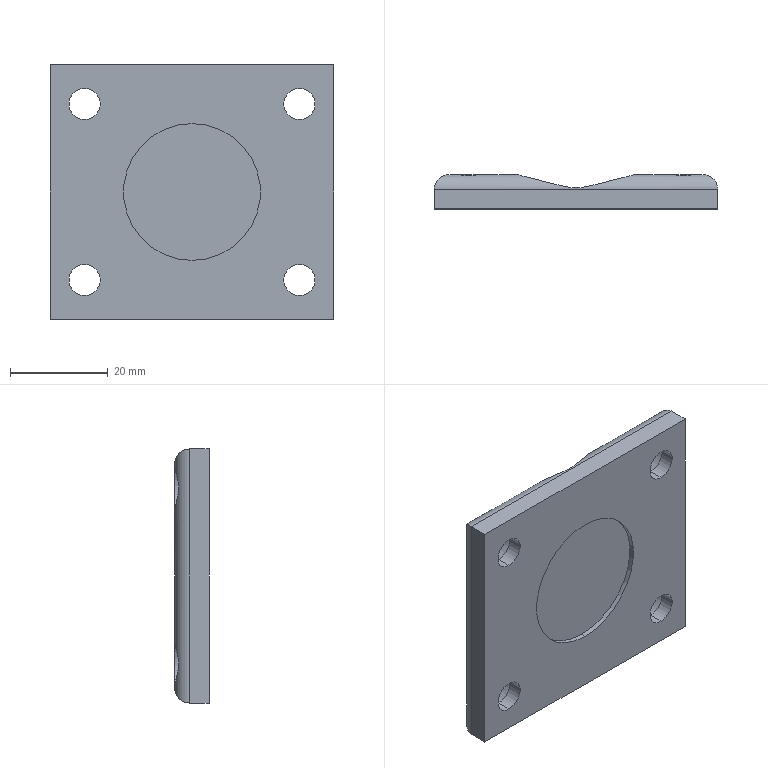Part | NX | features BREP 1 | 1 solid | 41 faces | box 58 x 7 x 52 mm | volume 16120 mm3 | cylinder 23 | plane 18 | commonest cylinder face diameters 6.4 x8 12 x8 6 x4 28 x2 20 x1
STEP:
#1=CARTESIAN_POINT('',(0.,204.,14.));
#2=VERTEX_POINT('',#1);
#3=CARTESIAN_POINT('',(0.,204.,-14.));
#4=VERTEX_POINT('',#3);
#5=CARTESIAN_POINT('',(0.,204.,0.));
#6=DIRECTION('',(0.,-1.,0.));
#7=DIRECTION('',(0.,0.,-1.));
#8=AXIS2_PLACEMENT_3D('',#5,#6,#7);
#9=CIRCLE('',#8,14.);
#10=EDGE_CURVE('',#2,#4,#9,.T.);
#11=ORIENTED_EDGE('',*,*,#10,.F.);
#12=CARTESIAN_POINT('',(0.,203.,14.));
#13=VERTEX_POINT('',#12);
#14=CARTESIAN_POINT('',(0.,204.,14.));
#15=DIRECTION('',(0.,-1.,0.));
#16=VECTOR('',#15,1000.);
#17=LINE('',#14,#16);
#18=EDGE_CURVE('',#2,#13,#17,.T.);
#19=ORIENTED_EDGE('',*,*,#18,.T.);
#20=CARTESIAN_POINT('',(0.,203.,-14.));
#21=VERTEX_POINT('',#20);
#22=CARTESIAN_POINT('',(0.,203.,0.));
#23=DIRECTION('',(0.,-1.,0.));
#24=DIRECTION('',(0.,0.,-1.));
#25=AXIS2_PLACEMENT_3D('',#22,#23,#24);
#26=CIRCLE('',#25,14.);
#27=EDGE_CURVE('',#13,#21,#26,.T.);
#28=ORIENTED_EDGE('',*,*,#27,.T.);
#29=CARTESIAN_POINT('',(0.,204.,-14.));
#30=DIRECTION('',(0.,1.,0.));
#31=VECTOR('',#30,1000.);
#32=LINE('',#29,#31);
#33=EDGE_CURVE('',#21,#4,#32,.T.);
#34=ORIENTED_EDGE('',*,*,#33,.T.);
#35=EDGE_LOOP('',(#11,#19,#28,#34));
#36=FACE_BOUND('',#35,.T.);
#37=CARTESIAN_POINT('',(0.,204.,0.));
#38=DIRECTION('',(0.,-1.,0.));
#39=DIRECTION('',(0.,0.,1.));
#40=AXIS2_PLACEMENT_3D('',#37,#38,#39);
#41=CYLINDRICAL_SURFACE('',#40,14.);
#42=ADVANCED_FACE('',(#36),#41,.F.);
#43=CARTESIAN_POINT('',(-22.,206.,-24.));
#44=VERTEX_POINT('',#43);
#45=CARTESIAN_POINT('',(-22.,206.,-12.));
#46=VERTEX_POINT('',#45);
#47=CARTESIAN_POINT('',(-22.,206.,-18.));
#48=DIRECTION('',(0.,1.,0.));
#49=DIRECTION('',(0.,0.,1.));
#50=AXIS2_PLACEMENT_3D('',#47,#48,#49);
#51=CIRCLE('',#50,6.);
#52=EDGE_CURVE('',#44,#46,#51,.T.);
#53=ORIENTED_EDGE('',*,*,#52,.F.);
#54=CARTESIAN_POINT('',(-22.,209.828,-24.));
#55=VERTEX_POINT('',#54);
#56=CARTESIAN_POINT('',(-22.,206.,-24.));
#57=DIRECTION('',(0.,1.,0.));
#58=VECTOR('',#57,1000.);
#59=LINE('',#56,#58);
#60=EDGE_CURVE('',#44,#55,#59,.T.);
#61=ORIENTED_EDGE('',*,*,#60,.T.);
#62=CARTESIAN_POINT('',(-25.317,210.,-23.));
#63=VERTEX_POINT('',#62);
#64=CARTESIAN_POINT('',(-22.,209.828,-24.));
#65=CARTESIAN_POINT('',(-23.183,209.828,-24.));
#66=CARTESIAN_POINT('',(-24.331,210.,-23.654));
#67=CARTESIAN_POINT('',(-25.317,210.,-23.));
#68=B_SPLINE_CURVE_WITH_KNOTS('',3,(#64,#65,#66,#67),.UNSPECIFIED.,.F.,.F.,(4,4),(0.,0.003498),.UNSPECIFIED.);
#69=EDGE_CURVE('',#55,#63,#68,.T.);
#70=ORIENTED_EDGE('',*,*,#69,.T.);
#71=CARTESIAN_POINT('',(-26.,210.,-22.472));
#72=VERTEX_POINT('',#71);
#73=CARTESIAN_POINT('',(-22.,210.,-18.));
#74=DIRECTION('',(0.,1.,0.));
#75=DIRECTION('',(0.,0.,1.));
#76=AXIS2_PLACEMENT_3D('',#73,#74,#75);
#77=CIRCLE('',#76,6.);
#78=EDGE_CURVE('',#63,#72,#77,.T.);
#79=ORIENTED_EDGE('',*,*,#78,.T.);
#80=CARTESIAN_POINT('',(-26.,210.,-13.528));
#81=VERTEX_POINT('',#80);
#82=CARTESIAN_POINT('',(-26.,210.,-22.472));
#83=CARTESIAN_POINT('',(-26.643,210.,-21.897));
#84=CARTESIAN_POINT('',(-27.633,209.605,-20.529));
#85=CARTESIAN_POINT('',(-28.183,209.052,-18.004));
#86=CARTESIAN_POINT('',(-27.634,209.604,-15.471));
#87=CARTESIAN_POINT('',(-26.642,210.,-14.102));
#88=CARTESIAN_POINT('',(-26.,210.,-13.528));
#89=B_SPLINE_CURVE_WITH_KNOTS('',3,(#82,#83,#84,#85,#86,#87,#88),.UNSPECIFIED.,.F.,.F.,(4,1,1,1,4),(0.,0.00255,0.0051,0.00765,0.0102),.UNSPECIFIED.);
#90=EDGE_CURVE('',#72,#81,#89,.T.);
#91=ORIENTED_EDGE('',*,*,#90,.T.);
#92=CARTESIAN_POINT('',(-22.,210.,-12.));
#93=VERTEX_POINT('',#92);
#94=CARTESIAN_POINT('',(-22.,210.,-18.));
#95=DIRECTION('',(0.,1.,0.));
#96=DIRECTION('',(0.,0.,1.));
#97=AXIS2_PLACEMENT_3D('',#94,#95,#96);
#98=CIRCLE('',#97,6.);
#99=EDGE_CURVE('',#81,#93,#98,.T.);
#100=ORIENTED_EDGE('',*,*,#99,.T.);
#101=CARTESIAN_POINT('',(-22.,206.,-12.));
#102=DIRECTION('',(0.,-1.,0.));
#103=VECTOR('',#102,1000.);
#104=LINE('',#101,#103);
#105=EDGE_CURVE('',#93,#46,#104,.T.);
#106=ORIENTED_EDGE('',*,*,#105,.T.);
#107=EDGE_LOOP('',(#53,#61,#70,#79,#91,#100,#106));
#108=FACE_BOUND('',#107,.T.);
#109=CARTESIAN_POINT('',(-22.,206.,-18.));
#110=DIRECTION('',(0.,1.,0.));
#111=DIRECTION('',(0.,0.,-1.));
#112=AXIS2_PLACEMENT_3D('',#109,#110,#111);
#113=CYLINDRICAL_SURFACE('',#112,6.);
#114=ADVANCED_FACE('',(#108),#113,.F.);
#115=CARTESIAN_POINT('',(22.,206.,-24.));
#116=VERTEX_POINT('',#115);
#117=CARTESIAN_POINT('',(22.,206.,-12.));
#118=VERTEX_POINT('',#117);
#119=CARTESIAN_POINT('',(22.,206.,-18.));
#120=DIRECTION('',(0.,1.,0.));
#121=DIRECTION('',(0.,0.,1.));
#122=AXIS2_PLACEMENT_3D('',#119,#120,#121);
#123=CIRCLE('',#122,6.);
#124=EDGE_CURVE('',#116,#118,#123,.T.);
#125=ORIENTED_EDGE('',*,*,#124,.F.);
#126=CARTESIAN_POINT('',(22.,209.828,-24.));
#127=VERTEX_POINT('',#126);
#128=CARTESIAN_POINT('',(22.,206.,-24.));
#129=DIRECTION('',(0.,-1.,0.));
#130=VECTOR('',#129,1000.);
#131=LINE('',#128,#130);
#132=EDGE_CURVE('',#127,#116,#131,.T.);
#133=ORIENTED_EDGE('',*,*,#132,.F.);
#134=CARTESIAN_POINT('',(18.683,210.,-23.));
#135=VERTEX_POINT('',#134);
#136=CARTESIAN_POINT('',(22.,209.828,-24.));
#137=CARTESIAN_POINT('',(20.817,209.828,-24.));
#138=CARTESIAN_POINT('',(19.669,210.,-23.654));
#139=CARTESIAN_POINT('',(18.683,210.,-23.));
#140=B_SPLINE_CURVE_WITH_KNOTS('',3,(#136,#137,#138,#139),.UNSPECIFIED.,.F.,.F.,(4,4),(0.,0.003498),.UNSPECIFIED.);
#141=EDGE_CURVE('',#127,#135,#140,.T.);
#142=ORIENTED_EDGE('',*,*,#141,.T.);
#143=CARTESIAN_POINT('',(22.,210.,-12.));
#144=VERTEX_POINT('',#143);
#145=CARTESIAN_POINT('',(22.,210.,-18.));
#146=DIRECTION('',(0.,1.,0.));
#147=DIRECTION('',(0.,0.,1.));
#148=AXIS2_PLACEMENT_3D('',#145,#146,#147);
#149=CIRCLE('',#148,6.);
#150=EDGE_CURVE('',#135,#144,#149,.T.);
#151=ORIENTED_EDGE('',*,*,#150,.T.);
#152=CARTESIAN_POINT('',(22.,206.,-12.));
#153=DIRECTION('',(0.,1.,0.));
#154=VECTOR('',#153,1000.);
#155=LINE('',#152,#154);
#156=EDGE_CURVE('',#118,#144,#155,.T.);
#157=ORIENTED_EDGE('',*,*,#156,.F.);
#158=EDGE_LOOP('',(#125,#133,#142,#151,#157));
#159=FACE_BOUND('',#158,.T.);
#160=CARTESIAN_POINT('',(22.,206.,-18.));
#161=DIRECTION('',(0.,1.,0.));
#162=DIRECTION('',(0.,0.,-1.));
#163=AXIS2_PLACEMENT_3D('',#160,#161,#162);
#164=CYLINDRICAL_SURFACE('',#163,6.);
#165=ADVANCED_FACE('',(#159),#164,.F.);
#166=CARTESIAN_POINT('',(22.,206.,12.));
#167=VERTEX_POINT('',#166);
#168=CARTESIAN_POINT('',(22.,206.,24.));
#169=VERTEX_POINT('',#168);
#170=CARTESIAN_POINT('',(22.,206.,18.));
#171=DIRECTION('',(0.,1.,0.));
#172=DIRECTION('',(0.,0.,1.));
#173=AXIS2_PLACEMENT_3D('',#170,#171,#172);
#174=CIRCLE('',#173,6.);
#175=EDGE_CURVE('',#167,#169,#174,.T.);
#176=ORIENTED_EDGE('',*,*,#175,.F.);
#177=CARTESIAN_POINT('',(22.,210.,12.));
#178=VERTEX_POINT('',#177);
#179=CARTESIAN_POINT('',(22.,206.,12.));
#180=DIRECTION('',(0.,1.,0.));
#181=VECTOR('',#180,1000.);
#182=LINE('',#179,#181);
#183=EDGE_CURVE('',#167,#178,#182,.T.);
#184=ORIENTED_EDGE('',*,*,#183,.T.);
#185=CARTESIAN_POINT('',(18.683,210.,23.));
#186=VERTEX_POINT('',#185);
#187=CARTESIAN_POINT('',(22.,210.,18.));
#188=DIRECTION('',(0.,1.,0.));
#189=DIRECTION('',(0.,0.,1.));
#190=AXIS2_PLACEMENT_3D('',#187,#188,#189);
#191=CIRCLE('',#190,6.);
#192=EDGE_CURVE('',#178,#186,#191,.T.);
#193=ORIENTED_EDGE('',*,*,#192,.T.);
#194=CARTESIAN_POINT('',(22.,209.828,24.));
#195=VERTEX_POINT('',#194);
#196=CARTESIAN_POINT('',(18.683,210.,23.));
#197=CARTESIAN_POINT('',(19.67,210.,23.654));
#198=CARTESIAN_POINT('',(20.818,209.828,24.));
#199=CARTESIAN_POINT('',(22.,209.828,24.));
#200=B_SPLINE_CURVE_WITH_KNOTS('',3,(#196,#197,#198,#199),.UNSPECIFIED.,.F.,.F.,(4,4),(0.,0.003499),.UNSPECIFIED.);
#201=EDGE_CURVE('',#186,#195,#200,.T.);
#202=ORIENTED_EDGE('',*,*,#201,.T.);
#203=CARTESIAN_POINT('',(22.,206.,24.));
#204=DIRECTION('',(0.,-1.,0.));
#205=VECTOR('',#204,1000.);
#206=LINE('',#203,#205);
#207=EDGE_CURVE('',#195,#169,#206,.T.);
#208=ORIENTED_EDGE('',*,*,#207,.T.);
#209=EDGE_LOOP('',(#176,#184,#193,#202,#208));
#210=FACE_BOUND('',#209,.T.);
#211=CARTESIAN_POINT('',(22.,206.,18.));
#212=DIRECTION('',(0.,1.,0.));
#213=DIRECTION('',(0.,0.,-1.));
#214=AXIS2_PLACEMENT_3D('',#211,#212,#213);
#215=CYLINDRICAL_SURFACE('',#214,6.);
#216=ADVANCED_FACE('',(#210),#215,.F.);
#217=CARTESIAN_POINT('',(-22.,206.,12.));
#218=VERTEX_POINT('',#217);
#219=CARTESIAN_POINT('',(-22.,206.,24.));
#220=VERTEX_POINT('',#219);
#221=CARTESIAN_POINT('',(-22.,206.,18.));
#222=DIRECTION('',(0.,1.,0.));
#223=DIRECTION('',(0.,0.,1.));
#224=AXIS2_PLACEMENT_3D('',#221,#222,#223);
#225=CIRCLE('',#224,6.);
#226=EDGE_CURVE('',#218,#220,#225,.T.);
#227=ORIENTED_EDGE('',*,*,#226,.F.);
#228=CARTESIAN_POINT('',(-22.,210.,12.));
#229=VERTEX_POINT('',#228);
#230=CARTESIAN_POINT('',(-22.,206.,12.));
#231=DIRECTION('',(0.,1.,0.));
#232=VECTOR('',#231,1000.);
#233=LINE('',#230,#232);
#234=EDGE_CURVE('',#218,#229,#233,.T.);
#235=ORIENTED_EDGE('',*,*,#234,.T.);
#236=CARTESIAN_POINT('',(-26.,210.,13.528));
#237=VERTEX_POINT('',#236);
#238=CARTESIAN_POINT('',(-22.,210.,18.));
#239=DIRECTION('',(0.,1.,0.));
#240=DIRECTION('',(0.,0.,1.));
#241=AXIS2_PLACEMENT_3D('',#238,#239,#240);
#242=CIRCLE('',#241,6.);
#243=EDGE_CURVE('',#229,#237,#242,.T.);
#244=ORIENTED_EDGE('',*,*,#243,.T.);
#245=CARTESIAN_POINT('',(-26.,210.,22.472));
#246=VERTEX_POINT('',#245);
#247=CARTESIAN_POINT('',(-26.,210.,13.528));
#248=CARTESIAN_POINT('',(-26.643,210.,14.103));
#249=CARTESIAN_POINT('',(-27.633,209.605,15.471));
#250=CARTESIAN_POINT('',(-28.183,209.052,17.996));
#251=CARTESIAN_POINT('',(-27.634,209.604,20.529));
#252=CARTESIAN_POINT('',(-26.642,210.,21.898));
#253=CARTESIAN_POINT('',(-26.,210.,22.472));
#254=B_SPLINE_CURVE_WITH_KNOTS('',3,(#247,#248,#249,#250,#251,#252,#253),.UNSPECIFIED.,.F.,.F.,(4,1,1,1,4),(0.,0.00255,0.0051,0.00765,0.0102),.UNSPECIFIED.);
#255=EDGE_CURVE('',#237,#246,#254,.T.);
#256=ORIENTED_EDGE('',*,*,#255,.T.);
#257=CARTESIAN_POINT('',(-25.317,210.,23.));
#258=VERTEX_POINT('',#257);
#259=CARTESIAN_POINT('',(-22.,210.,18.));
#260=DIRECTION('',(0.,1.,0.));
#261=DIRECTION('',(0.,0.,1.));
#262=AXIS2_PLACEMENT_3D('',#259,#260,#261);
#263=CIRCLE('',#262,6.);
#264=EDGE_CURVE('',#246,#258,#263,.T.);
#265=ORIENTED_EDGE('',*,*,#264,.T.);
#266=CARTESIAN_POINT('',(-22.,209.828,24.));
#267=VERTEX_POINT('',#266);
#268=CARTESIAN_POINT('',(-25.317,210.,23.));
#269=CARTESIAN_POINT('',(-24.33,210.,23.654));
#270=CARTESIAN_POINT('',(-23.182,209.828,24.));
#271=CARTESIAN_POINT('',(-22.,209.828,24.));
#272=B_SPLINE_CURVE_WITH_KNOTS('',3,(#268,#269,#270,#271),.UNSPECIFIED.,.F.,.F.,(4,4),(0.,0.003499),.UNSPECIFIED.);
#273=EDGE_CURVE('',#258,#267,#272,.T.);
#274=ORIENTED_EDGE('',*,*,#273,.T.);
#275=CARTESIAN_POINT('',(-22.,206.,24.));
#276=DIRECTION('',(0.,-1.,0.));
#277=VECTOR('',#276,1000.);
#278=LINE('',#275,#277);
#279=EDGE_CURVE('',#267,#220,#278,.T.);
#280=ORIENTED_EDGE('',*,*,#279,.T.);
#281=EDGE_LOOP('',(#227,#235,#244,#256,#265,#274,#280));
#282=FACE_BOUND('',#281,.T.);
#283=CARTESIAN_POINT('',(-22.,206.,18.));
#284=DIRECTION('',(0.,1.,0.));
#285=DIRECTION('',(0.,0.,-1.));
#286=AXIS2_PLACEMENT_3D('',#283,#284,#285);
#287=CYLINDRICAL_SURFACE('',#286,6.);
#288=ADVANCED_FACE('',(#282),#287,.F.);
#289=CARTESIAN_POINT('',(-22.,206.,14.8));
#290=VERTEX_POINT('',#289);
#291=CARTESIAN_POINT('',(-22.,206.,21.2));
#292=VERTEX_POINT('',#291);
#293=CARTESIAN_POINT('',(-22.,206.,18.));
#294=DIRECTION('',(0.,1.,0.));
#295=DIRECTION('',(0.,0.,1.));
#296=AXIS2_PLACEMENT_3D('',#293,#294,#295);
#297=CIRCLE('',#296,3.2);
#298=EDGE_CURVE('',#290,#292,#297,.T.);
#299=ORIENTED_EDGE('',*,*,#298,.T.);
#300=CARTESIAN_POINT('',(-22.,203.,21.2));
#301=VERTEX_POINT('',#300);
#302=CARTESIAN_POINT('',(-22.,210.,21.2));
#303=DIRECTION('',(0.,-1.,0.));
#304=VECTOR('',#303,1000.);
#305=LINE('',#302,#304);
#306=EDGE_CURVE('',#292,#301,#305,.T.);
#307=ORIENTED_EDGE('',*,*,#306,.T.);
#308=CARTESIAN_POINT('',(-22.,203.,14.8));
#309=VERTEX_POINT('',#308);
#310=CARTESIAN_POINT('',(-22.,203.,18.));
#311=DIRECTION('',(0.,1.,0.));
#312=DIRECTION('',(0.,0.,-1.));
#313=AXIS2_PLACEMENT_3D('',#310,#311,#312);
#314=CIRCLE('',#313,3.2);
#315=EDGE_CURVE('',#309,#301,#314,.T.);
#316=ORIENTED_EDGE('',*,*,#315,.F.);
#317=CARTESIAN_POINT('',(-22.,210.,14.8));
#318=DIRECTION('',(0.,1.,0.));
#319=VECTOR('',#318,1000.);
#320=LINE('',#317,#319);
#321=EDGE_CURVE('',#309,#290,#320,.T.);
#322=ORIENTED_EDGE('',*,*,#321,.T.);
#323=EDGE_LOOP('',(#299,#307,#316,#322));
#324=FACE_BOUND('',#323,.T.);
#325=CARTESIAN_POINT('',(-22.,210.,18.));
#326=DIRECTION('',(0.,-1.,0.));
#327=DIRECTION('',(0.,0.,1.));
#328=AXIS2_PLACEMENT_3D('',#325,#326,#327);
#329=CYLINDRICAL_SURFACE('',#328,3.2);
#330=ADVANCED_FACE('',(#324),#329,.F.);
#331=CARTESIAN_POINT('',(22.,206.,14.8));
#332=VERTEX_POINT('',#331);
#333=CARTESIAN_POINT('',(22.,206.,21.2));
#334=VERTEX_POINT('',#333);
#335=CARTESIAN_POINT('',(22.,206.,18.));
#336=DIRECTION('',(0.,1.,0.));
#337=DIRECTION('',(0.,0.,1.));
#338=AXIS2_PLACEMENT_3D('',#335,#336,#337);
#339=CIRCLE('',#338,3.2);
#340=EDGE_CURVE('',#332,#334,#339,.T.);
#341=ORIENTED_EDGE('',*,*,#340,.T.);
#342=CARTESIAN_POINT('',(22.,203.,21.2));
#343=VERTEX_POINT('',#342);
#344=CARTESIAN_POINT('',(22.,210.,21.2));
#345=DIRECTION('',(0.,1.,0.));
#346=VECTOR('',#345,1000.);
#347=LINE('',#344,#346);
#348=EDGE_CURVE('',#343,#334,#347,.T.);
#349=ORIENTED_EDGE('',*,*,#348,.F.);
#350=CARTESIAN_POINT('',(22.,203.,14.8));
#351=VERTEX_POINT('',#350);
#352=CARTESIAN_POINT('',(22.,203.,18.));
#353=DIRECTION('',(0.,1.,0.));
#354=DIRECTION('',(0.,0.,1.));
#355=AXIS2_PLACEMENT_3D('',#352,#353,#354);
#356=CIRCLE('',#355,3.2);
#357=EDGE_CURVE('',#351,#343,#356,.T.);
#358=ORIENTED_EDGE('',*,*,#357,.F.);
#359=CARTESIAN_POINT('',(22.,210.,14.8));
#360=DIRECTION('',(0.,-1.,0.));
#361=VECTOR('',#360,1000.);
#362=LINE('',#359,#361);
#363=EDGE_CURVE('',#332,#351,#362,.T.);
#364=ORIENTED_EDGE('',*,*,#363,.F.);
#365=EDGE_LOOP('',(#341,#349,#358,#364));
#366=FACE_BOUND('',#365,.T.);
#367=CARTESIAN_POINT('',(22.,210.,18.));
#368=DIRECTION('',(0.,-1.,0.));
#369=DIRECTION('',(0.,0.,1.));
#370=AXIS2_PLACEMENT_3D('',#367,#368,#369);
#371=CYLINDRICAL_SURFACE('',#370,3.2);
#372=ADVANCED_FACE('',(#366),#371,.F.);
#373=CARTESIAN_POINT('',(22.,206.,-21.2));
#374=VERTEX_POINT('',#373);
#375=CARTESIAN_POINT('',(22.,206.,-14.8));
#376=VERTEX_POINT('',#375);
#377=CARTESIAN_POINT('',(22.,206.,-18.));
#378=DIRECTION('',(0.,1.,0.));
#379=DIRECTION('',(0.,0.,1.));
#380=AXIS2_PLACEMENT_3D('',#377,#378,#379);
#381=CIRCLE('',#380,3.2);
#382=EDGE_CURVE('',#374,#376,#381,.T.);
#383=ORIENTED_EDGE('',*,*,#382,.T.);
#384=CARTESIAN_POINT('',(22.,203.,-14.8));
#385=VERTEX_POINT('',#384);
#386=CARTESIAN_POINT('',(22.,210.,-14.8));
#387=DIRECTION('',(0.,-1.,0.));
#388=VECTOR('',#387,1000.);
#389=LINE('',#386,#388);
#390=EDGE_CURVE('',#376,#385,#389,.T.);
#391=ORIENTED_EDGE('',*,*,#390,.T.);
#392=CARTESIAN_POINT('',(22.,203.,-21.2));
#393=VERTEX_POINT('',#392);
#394=CARTESIAN_POINT('',(22.,203.,-18.));
#395=DIRECTION('',(0.,1.,0.));
#396=DIRECTION('',(0.,0.,-1.));
#397=AXIS2_PLACEMENT_3D('',#394,#395,#396);
#398=CIRCLE('',#397,3.2);
#399=EDGE_CURVE('',#393,#385,#398,.T.);
#400=ORIENTED_EDGE('',*,*,#399,.F.);
#401=CARTESIAN_POINT('',(22.,210.,-21.2));
#402=DIRECTION('',(0.,1.,0.));
#403=VECTOR('',#402,1000.);
#404=LINE('',#401,#403);
#405=EDGE_CURVE('',#393,#374,#404,.T.);
#406=ORIENTED_EDGE('',*,*,#405,.T.);
#407=EDGE_LOOP('',(#383,#391,#400,#406));
#408=FACE_BOUND('',#407,.T.);
#409=CARTESIAN_POINT('',(22.,210.,-18.));
#410=DIRECTION('',(0.,-1.,0.));
#411=DIRECTION('',(0.,0.,1.));
#412=AXIS2_PLACEMENT_3D('',#409,#410,#411);
#413=CYLINDRICAL_SURFACE('',#412,3.2);
#414=ADVANCED_FACE('',(#408),#413,.F.);
#415=CARTESIAN_POINT('',(-22.,206.,-21.2));
#416=VERTEX_POINT('',#415);
#417=CARTESIAN_POINT('',(-22.,206.,-14.8));
#418=VERTEX_POINT('',#417);
#419=CARTESIAN_POINT('',(-22.,206.,-18.));
#420=DIRECTION('',(0.,1.,0.));
#421=DIRECTION('',(0.,0.,1.));
#422=AXIS2_PLACEMENT_3D('',#419,#420,#421);
#423=CIRCLE('',#422,3.2);
#424=EDGE_CURVE('',#416,#418,#423,.T.);
#425=ORIENTED_EDGE('',*,*,#424,.T.);
#426=CARTESIAN_POINT('',(-22.,203.,-14.8));
#427=VERTEX_POINT('',#426);
#428=CARTESIAN_POINT('',(-22.,210.,-14.8));
#429=DIRECTION('',(0.,1.,0.));
#430=VECTOR('',#429,1000.);
#431=LINE('',#428,#430);
#432=EDGE_CURVE('',#427,#418,#431,.T.);
#433=ORIENTED_EDGE('',*,*,#432,.F.);
#434=CARTESIAN_POINT('',(-22.,203.,-21.2));
#435=VERTEX_POINT('',#434);
#436=CARTESIAN_POINT('',(-22.,203.,-18.));
#437=DIRECTION('',(0.,1.,0.));
#438=DIRECTION('',(0.,0.,1.));
#439=AXIS2_PLACEMENT_3D('',#436,#437,#438);
#440=CIRCLE('',#439,3.2);
#441=EDGE_CURVE('',#435,#427,#440,.T.);
#442=ORIENTED_EDGE('',*,*,#441,.F.);
#443=CARTESIAN_POINT('',(-22.,210.,-21.2));
#444=DIRECTION('',(0.,-1.,0.));
#445=VECTOR('',#444,1000.);
#446=LINE('',#443,#445);
#447=EDGE_CURVE('',#416,#435,#446,.T.);
#448=ORIENTED_EDGE('',*,*,#447,.F.);
#449=EDGE_LOOP('',(#425,#433,#442,#448));
#450=FACE_BOUND('',#449,.T.);
#451=CARTESIAN_POINT('',(-22.,210.,-18.));
#452=DIRECTION('',(0.,-1.,0.));
#453=DIRECTION('',(0.,0.,1.));
#454=AXIS2_PLACEMENT_3D('',#451,#452,#453);
#455=CYLINDRICAL_SURFACE('',#454,3.2);
#456=ADVANCED_FACE('',(#450),#455,.F.);
#457=CARTESIAN_POINT('',(12.,210.,-23.));
#458=VERTEX_POINT('',#457);
#459=CARTESIAN_POINT('',(-29.,210.,-23.));
#460=DIRECTION('',(-1.,0.,0.));
#461=VECTOR('',#460,1000.);
#462=LINE('',#459,#461);
#463=EDGE_CURVE('',#135,#458,#462,.T.);
#464=ORIENTED_EDGE('',*,*,#463,.T.);
#465=CARTESIAN_POINT('',(12.,210.,23.));
#466=VERTEX_POINT('',#465);
#467=CARTESIAN_POINT('',(12.,210.,-28.));
#468=DIRECTION('',(0.,0.,1.));
#469=VECTOR('',#468,1000.);
#470=LINE('',#467,#469);
#471=EDGE_CURVE('',#458,#466,#470,.T.);
#472=ORIENTED_EDGE('',*,*,#471,.T.);
#473=CARTESIAN_POINT('',(-29.,210.,23.));
#474=DIRECTION('',(1.,0.,0.));
#475=VECTOR('',#474,1000.);
#476=LINE('',#473,#475);
#477=EDGE_CURVE('',#466,#186,#476,.T.);
#478=ORIENTED_EDGE('',*,*,#477,.T.);
#479=ORIENTED_EDGE('',*,*,#192,.F.);
#480=CARTESIAN_POINT('',(26.,210.,13.528));
#481=VERTEX_POINT('',#480);
#482=CARTESIAN_POINT('',(22.,210.,18.));
#483=DIRECTION('',(0.,1.,0.));
#484=DIRECTION('',(0.,0.,1.));
#485=AXIS2_PLACEMENT_3D('',#482,#483,#484);
#486=CIRCLE('',#485,6.);
#487=EDGE_CURVE('',#481,#178,#486,.T.);
#488=ORIENTED_EDGE('',*,*,#487,.F.);
#489=CARTESIAN_POINT('',(26.,210.,-13.528));
#490=VERTEX_POINT('',#489);
#491=CARTESIAN_POINT('',(26.,210.,26.));
#492=DIRECTION('',(0.,0.,-1.));
#493=VECTOR('',#492,1000.);
#494=LINE('',#491,#493);
#495=EDGE_CURVE('',#481,#490,#494,.T.);
#496=ORIENTED_EDGE('',*,*,#495,.T.);
#497=CARTESIAN_POINT('',(22.,210.,-18.));
#498=DIRECTION('',(0.,1.,0.));
#499=DIRECTION('',(0.,0.,1.));
#500=AXIS2_PLACEMENT_3D('',#497,#498,#499);
#501=CIRCLE('',#500,6.);
#502=EDGE_CURVE('',#144,#490,#501,.T.);
#503=ORIENTED_EDGE('',*,*,#502,.F.);
#504=ORIENTED_EDGE('',*,*,#150,.F.);
#505=EDGE_LOOP('',(#464,#472,#478,#479,#488,#496,#503,#504));
#506=FACE_BOUND('',#505,.T.);
#507=CARTESIAN_POINT('',(-29.,210.,26.));
#508=DIRECTION('',(0.,-1.,0.));
#509=DIRECTION('',(0.,0.,1.));
#510=AXIS2_PLACEMENT_3D('',#507,#508,#509);
#511=PLANE('',#510);
#512=ADVANCED_FACE('',(#506),#511,.F.);
#513=CARTESIAN_POINT('',(2.425,207.606,25.938));
#514=VERTEX_POINT('',#513);
#515=CARTESIAN_POINT('',(2.425,207.606,25.938));
#516=CARTESIAN_POINT('',(8.246,209.062,25.638));
#517=CARTESIAN_POINT('',(12.,210.,24.486));
#518=CARTESIAN_POINT('',(12.,210.,23.));
#519=(BOUNDED_CURVE()B_SPLINE_CURVE(3,(#515,#516,#517,#518),.UNSPECIFIED.,.F.,.F.)B_SPLINE_CURVE_WITH_KNOTS((4,4),(0.,1.),.PIECEWISE_BEZIER_KNOTS.)CURVE()GEOMETRIC_REPRESENTATION_ITEM()RATIONAL_B_SPLINE_CURVE((1.,0.8502,0.8502,1.))REPRESENTATION_ITEM(''));
#520=EDGE_CURVE('',#514,#466,#519,.T.);
#521=ORIENTED_EDGE('',*,*,#520,.F.);
#522=CARTESIAN_POINT('',(-2.425,207.606,25.938));
#523=VERTEX_POINT('',#522);
#524=CARTESIAN_POINT('',(2.425,207.606,25.938));
#525=CARTESIAN_POINT('',(0.8323,207.208,26.02));
#526=CARTESIAN_POINT('',(-0.8326,207.208,26.02));
#527=CARTESIAN_POINT('',(-2.425,207.606,25.938));
#528=B_SPLINE_CURVE_WITH_KNOTS('',3,(#524,#525,#526,#527),.UNSPECIFIED.,.F.,.F.,(4,4),(0.,0.004872),.UNSPECIFIED.);
#529=EDGE_CURVE('',#514,#523,#528,.T.);
#530=ORIENTED_EDGE('',*,*,#529,.T.);
#531=CARTESIAN_POINT('',(-12.,210.,23.));
#532=VERTEX_POINT('',#531);
#533=CARTESIAN_POINT('',(-12.,210.,23.));
#534=CARTESIAN_POINT('',(-12.,210.,24.486));
#535=CARTESIAN_POINT('',(-8.246,209.062,25.638));
#536=CARTESIAN_POINT('',(-2.425,207.606,25.938));
#537=(BOUNDED_CURVE()B_SPLINE_CURVE(3,(#533,#534,#535,#536),.UNSPECIFIED.,.F.,.F.)B_SPLINE_CURVE_WITH_KNOTS((4,4),(0.,1.),.PIECEWISE_BEZIER_KNOTS.)CURVE()GEOMETRIC_REPRESENTATION_ITEM()RATIONAL_B_SPLINE_CURVE((1.,0.8502,0.8502,1.))REPRESENTATION_ITEM(''));
#538=EDGE_CURVE('',#532,#523,#537,.T.);
#539=ORIENTED_EDGE('',*,*,#538,.F.);
#540=CARTESIAN_POINT('',(-18.683,210.,23.));
#541=VERTEX_POINT('',#540);
#542=CARTESIAN_POINT('',(-29.,210.,23.));
#543=DIRECTION('',(1.,0.,0.));
#544=VECTOR('',#543,1000.);
#545=LINE('',#542,#544);
#546=EDGE_CURVE('',#541,#532,#545,.T.);
#547=ORIENTED_EDGE('',*,*,#546,.F.);
#548=CARTESIAN_POINT('',(-22.,209.828,24.));
#549=CARTESIAN_POINT('',(-20.817,209.828,24.));
#550=CARTESIAN_POINT('',(-19.669,210.,23.654));
#551=CARTESIAN_POINT('',(-18.683,210.,23.));
#552=B_SPLINE_CURVE_WITH_KNOTS('',3,(#548,#549,#550,#551),.UNSPECIFIED.,.F.,.F.,(4,4),(0.,0.003498),.UNSPECIFIED.);
#553=EDGE_CURVE('',#267,#541,#552,.T.);
#554=ORIENTED_EDGE('',*,*,#553,.F.);
#555=ORIENTED_EDGE('',*,*,#273,.F.);
#556=CARTESIAN_POINT('',(-26.,210.,23.));
#557=VERTEX_POINT('',#556);
#558=CARTESIAN_POINT('',(-29.,210.,23.));
#559=DIRECTION('',(1.,0.,0.));
#560=VECTOR('',#559,1000.);
#561=LINE('',#558,#560);
#562=EDGE_CURVE('',#557,#258,#561,.T.);
#563=ORIENTED_EDGE('',*,*,#562,.F.);
#564=CARTESIAN_POINT('',(-29.,207.,26.));
#565=VERTEX_POINT('',#564);
#566=CARTESIAN_POINT('',(-29.,207.,26.));
#567=CARTESIAN_POINT('',(-29.,208.757,26.));
#568=CARTESIAN_POINT('',(-27.757,210.,24.757));
#569=CARTESIAN_POINT('',(-26.,210.,23.));
#570=(BOUNDED_CURVE()B_SPLINE_CURVE(3,(#566,#567,#568,#569),.UNSPECIFIED.,.F.,.F.)B_SPLINE_CURVE_WITH_KNOTS((4,4),(0.,1.),.PIECEWISE_BEZIER_KNOTS.)CURVE()GEOMETRIC_REPRESENTATION_ITEM()RATIONAL_B_SPLINE_CURVE((1.,0.8047,0.8047,1.))REPRESENTATION_ITEM(''));
#571=EDGE_CURVE('',#565,#557,#570,.T.);
#572=ORIENTED_EDGE('',*,*,#571,.F.);
#573=CARTESIAN_POINT('',(29.,207.,26.));
#574=VERTEX_POINT('',#573);
#575=CARTESIAN_POINT('',(-29.,207.,26.));
#576=DIRECTION('',(-1.,0.,0.));
#577=VECTOR('',#576,1000.);
#578=LINE('',#575,#577);
#579=EDGE_CURVE('',#574,#565,#578,.T.);
#580=ORIENTED_EDGE('',*,*,#579,.F.);
#581=CARTESIAN_POINT('',(26.,210.,23.));
#582=VERTEX_POINT('',#581);
#583=CARTESIAN_POINT('',(26.,210.,23.));
#584=CARTESIAN_POINT('',(27.757,210.,24.757));
#585=CARTESIAN_POINT('',(29.,208.757,26.));
#586=CARTESIAN_POINT('',(29.,207.,26.));
#587=(BOUNDED_CURVE()B_SPLINE_CURVE(3,(#583,#584,#585,#586),.UNSPECIFIED.,.F.,.F.)B_SPLINE_CURVE_WITH_KNOTS((4,4),(0.,1.),.PIECEWISE_BEZIER_KNOTS.)CURVE()GEOMETRIC_REPRESENTATION_ITEM()RATIONAL_B_SPLINE_CURVE((1.,0.8047,0.8047,1.))REPRESENTATION_ITEM(''));
#588=EDGE_CURVE('',#582,#574,#587,.T.);
#589=ORIENTED_EDGE('',*,*,#588,.F.);
#590=CARTESIAN_POINT('',(25.317,210.,23.));
#591=VERTEX_POINT('',#590);
#592=CARTESIAN_POINT('',(-29.,210.,23.));
#593=DIRECTION('',(1.,0.,0.));
#594=VECTOR('',#593,1000.);
#595=LINE('',#592,#594);
#596=EDGE_CURVE('',#591,#582,#595,.T.);
#597=ORIENTED_EDGE('',*,*,#596,.F.);
#598=CARTESIAN_POINT('',(22.,209.828,24.));
#599=CARTESIAN_POINT('',(23.183,209.828,24.));
#600=CARTESIAN_POINT('',(24.331,210.,23.654));
#601=CARTESIAN_POINT('',(25.317,210.,23.));
#602=B_SPLINE_CURVE_WITH_KNOTS('',3,(#598,#599,#600,#601),.UNSPECIFIED.,.F.,.F.,(4,4),(0.,0.003498),.UNSPECIFIED.);
#603=EDGE_CURVE('',#195,#591,#602,.T.);
#604=ORIENTED_EDGE('',*,*,#603,.F.);
#605=ORIENTED_EDGE('',*,*,#201,.F.);
#606=ORIENTED_EDGE('',*,*,#477,.F.);
#607=EDGE_LOOP('',(#521,#530,#539,#547,#554,#555,#563,#572,#580,#589,#597,#604,#605,#606));
#608=FACE_BOUND('',#607,.T.);
#609=CARTESIAN_POINT('',(-29.,207.,23.));
#610=DIRECTION('',(1.,0.,0.));
#611=DIRECTION('',(0.,0.,1.));
#612=AXIS2_PLACEMENT_3D('',#609,#610,#611);
#613=CYLINDRICAL_SURFACE('',#612,3.);
#614=ADVANCED_FACE('',(#608),#613,.T.);
#615=ORIENTED_EDGE('',*,*,#546,.T.);
#616=CARTESIAN_POINT('',(-12.,210.,-23.));
#617=VERTEX_POINT('',#616);
#618=CARTESIAN_POINT('',(-12.,210.,-28.));
#619=DIRECTION('',(0.,0.,1.));
#620=VECTOR('',#619,1000.);
#621=LINE('',#618,#620);
#622=EDGE_CURVE('',#617,#532,#621,.T.);
#623=ORIENTED_EDGE('',*,*,#622,.F.);
#624=CARTESIAN_POINT('',(-18.683,210.,-23.));
#625=VERTEX_POINT('',#624);
#626=CARTESIAN_POINT('',(-29.,210.,-23.));
#627=DIRECTION('',(-1.,0.,0.));
#628=VECTOR('',#627,1000.);
#629=LINE('',#626,#628);
#630=EDGE_CURVE('',#617,#625,#629,.T.);
#631=ORIENTED_EDGE('',*,*,#630,.T.);
#632=CARTESIAN_POINT('',(-22.,210.,-18.));
#633=DIRECTION('',(0.,1.,0.));
#634=DIRECTION('',(0.,0.,1.));
#635=AXIS2_PLACEMENT_3D('',#632,#633,#634);
#636=CIRCLE('',#635,6.);
#637=EDGE_CURVE('',#93,#625,#636,.T.);
#638=ORIENTED_EDGE('',*,*,#637,.F.);
#639=ORIENTED_EDGE('',*,*,#99,.F.);
#640=CARTESIAN_POINT('',(-26.,210.,26.));
#641=DIRECTION('',(0.,0.,1.));
#642=VECTOR('',#641,1000.);
#643=LINE('',#640,#642);
#644=EDGE_CURVE('',#81,#237,#643,.T.);
#645=ORIENTED_EDGE('',*,*,#644,.T.);
#646=ORIENTED_EDGE('',*,*,#243,.F.);
#647=CARTESIAN_POINT('',(-22.,210.,18.));
#648=DIRECTION('',(0.,1.,0.));
#649=DIRECTION('',(0.,0.,1.));
#650=AXIS2_PLACEMENT_3D('',#647,#648,#649);
#651=CIRCLE('',#650,6.);
#652=EDGE_CURVE('',#541,#229,#651,.T.);
#653=ORIENTED_EDGE('',*,*,#652,.F.);
#654=EDGE_LOOP('',(#615,#623,#631,#638,#639,#645,#646,#653));
#655=FACE_BOUND('',#654,.T.);
#656=CARTESIAN_POINT('',(-29.,210.,26.));
#657=DIRECTION('',(0.,-1.,0.));
#658=DIRECTION('',(0.,0.,1.));
#659=AXIS2_PLACEMENT_3D('',#656,#657,#658);
#660=PLANE('',#659);
#661=ADVANCED_FACE('',(#655),#660,.F.);
#662=CARTESIAN_POINT('',(26.,210.,-22.472));
#663=VERTEX_POINT('',#662);
#664=CARTESIAN_POINT('',(26.,210.,-23.));
#665=VERTEX_POINT('',#664);
#666=CARTESIAN_POINT('',(26.,210.,26.));
#667=DIRECTION('',(0.,0.,-1.));
#668=VECTOR('',#667,1000.);
#669=LINE('',#666,#668);
#670=EDGE_CURVE('',#663,#665,#669,.T.);
#671=ORIENTED_EDGE('',*,*,#670,.T.);
#672=CARTESIAN_POINT('',(25.317,210.,-23.));
#673=VERTEX_POINT('',#672);
#674=CARTESIAN_POINT('',(-29.,210.,-23.));
#675=DIRECTION('',(-1.,0.,0.));
#676=VECTOR('',#675,1000.);
#677=LINE('',#674,#676);
#678=EDGE_CURVE('',#665,#673,#677,.T.);
#679=ORIENTED_EDGE('',*,*,#678,.T.);
#680=CARTESIAN_POINT('',(22.,210.,-18.));
#681=DIRECTION('',(0.,1.,0.));
#682=DIRECTION('',(0.,0.,1.));
#683=AXIS2_PLACEMENT_3D('',#680,#681,#682);
#684=CIRCLE('',#683,6.);
#685=EDGE_CURVE('',#663,#673,#684,.T.);
#686=ORIENTED_EDGE('',*,*,#685,.F.);
#687=EDGE_LOOP('',(#671,#679,#686));
#688=FACE_BOUND('',#687,.T.);
#689=CARTESIAN_POINT('',(-29.,210.,26.));
#690=DIRECTION('',(0.,-1.,0.));
#691=DIRECTION('',(0.,0.,1.));
#692=AXIS2_PLACEMENT_3D('',#689,#690,#691);
#693=PLANE('',#692);
#694=ADVANCED_FACE('',(#688),#693,.F.);
#695=ORIENTED_EDGE('',*,*,#78,.F.);
#696=CARTESIAN_POINT('',(-26.,210.,-23.));
#697=VERTEX_POINT('',#696);
#698=CARTESIAN_POINT('',(-29.,210.,-23.));
#699=DIRECTION('',(-1.,0.,0.));
#700=VECTOR('',#699,1000.);
#701=LINE('',#698,#700);
#702=EDGE_CURVE('',#63,#697,#701,.T.);
#703=ORIENTED_EDGE('',*,*,#702,.T.);
#704=CARTESIAN_POINT('',(-26.,210.,26.));
#705=DIRECTION('',(0.,0.,1.));
#706=VECTOR('',#705,1000.);
#707=LINE('',#704,#706);
#708=EDGE_CURVE('',#697,#72,#707,.T.);
#709=ORIENTED_EDGE('',*,*,#708,.T.);
#710=EDGE_LOOP('',(#695,#703,#709));
#711=FACE_BOUND('',#710,.T.);
#712=CARTESIAN_POINT('',(-29.,210.,26.));
#713=DIRECTION('',(0.,-1.,0.));
#714=DIRECTION('',(0.,0.,1.));
#715=AXIS2_PLACEMENT_3D('',#712,#713,#714);
#716=PLANE('',#715);
#717=ADVANCED_FACE('',(#711),#716,.F.);
#718=ORIENTED_EDGE('',*,*,#264,.F.);
#719=CARTESIAN_POINT('',(-26.,210.,26.));
#720=DIRECTION('',(0.,0.,1.));
#721=VECTOR('',#720,1000.);
#722=LINE('',#719,#721);
#723=EDGE_CURVE('',#246,#557,#722,.T.);
#724=ORIENTED_EDGE('',*,*,#723,.T.);
#725=ORIENTED_EDGE('',*,*,#562,.T.);
#726=EDGE_LOOP('',(#718,#724,#725));
#727=FACE_BOUND('',#726,.T.);
#728=CARTESIAN_POINT('',(-29.,210.,26.));
#729=DIRECTION('',(0.,-1.,0.));
#730=DIRECTION('',(0.,0.,1.));
#731=AXIS2_PLACEMENT_3D('',#728,#729,#730);
#732=PLANE('',#731);
#733=ADVANCED_FACE('',(#727),#732,.F.);
#734=ORIENTED_EDGE('',*,*,#432,.T.);
#735=CARTESIAN_POINT('',(-22.,206.,-18.));
#736=DIRECTION('',(0.,1.,0.));
#737=DIRECTION('',(0.,0.,1.));
#738=AXIS2_PLACEMENT_3D('',#735,#736,#737);
#739=CIRCLE('',#738,3.2);
#740=EDGE_CURVE('',#418,#416,#739,.T.);
#741=ORIENTED_EDGE('',*,*,#740,.T.);
#742=ORIENTED_EDGE('',*,*,#447,.T.);
#743=CARTESIAN_POINT('',(-22.,203.,-18.));
#744=DIRECTION('',(0.,1.,0.));
#745=DIRECTION('',(0.,0.,1.));
#746=AXIS2_PLACEMENT_3D('',#743,#744,#745);
#747=CIRCLE('',#746,3.2);
#748=EDGE_CURVE('',#427,#435,#747,.T.);
#749=ORIENTED_EDGE('',*,*,#748,.F.);
#750=EDGE_LOOP('',(#734,#741,#742,#749));
#751=FACE_BOUND('',#750,.T.);
#752=CARTESIAN_POINT('',(-22.,210.,-18.));
#753=DIRECTION('',(0.,-1.,0.));
#754=DIRECTION('',(0.,0.,1.));
#755=AXIS2_PLACEMENT_3D('',#752,#753,#754);
#756=CYLINDRICAL_SURFACE('',#755,3.2);
#757=ADVANCED_FACE('',(#751),#756,.F.);
#758=ORIENTED_EDGE('',*,*,#390,.F.);
#759=CARTESIAN_POINT('',(22.,206.,-18.));
#760=DIRECTION('',(0.,1.,0.));
#761=DIRECTION('',(0.,0.,1.));
#762=AXIS2_PLACEMENT_3D('',#759,#760,#761);
#763=CIRCLE('',#762,3.2);
#764=EDGE_CURVE('',#376,#374,#763,.T.);
#765=ORIENTED_EDGE('',*,*,#764,.T.);
#766=ORIENTED_EDGE('',*,*,#405,.F.);
#767=CARTESIAN_POINT('',(22.,203.,-18.));
#768=DIRECTION('',(0.,1.,0.));
#769=DIRECTION('',(0.,0.,-1.));
#770=AXIS2_PLACEMENT_3D('',#767,#768,#769);
#771=CIRCLE('',#770,3.2);
#772=EDGE_CURVE('',#385,#393,#771,.T.);
#773=ORIENTED_EDGE('',*,*,#772,.F.);
#774=EDGE_LOOP('',(#758,#765,#766,#773));
#775=FACE_BOUND('',#774,.T.);
#776=CARTESIAN_POINT('',(22.,210.,-18.));
#777=DIRECTION('',(0.,-1.,0.));
#778=DIRECTION('',(0.,0.,1.));
#779=AXIS2_PLACEMENT_3D('',#776,#777,#778);
#780=CYLINDRICAL_SURFACE('',#779,3.2);
#781=ADVANCED_FACE('',(#775),#780,.F.);
#782=ORIENTED_EDGE('',*,*,#348,.T.);
#783=CARTESIAN_POINT('',(22.,206.,18.));
#784=DIRECTION('',(0.,1.,0.));
#785=DIRECTION('',(0.,0.,1.));
#786=AXIS2_PLACEMENT_3D('',#783,#784,#785);
#787=CIRCLE('',#786,3.2);
#788=EDGE_CURVE('',#334,#332,#787,.T.);
#789=ORIENTED_EDGE('',*,*,#788,.T.);
#790=ORIENTED_EDGE('',*,*,#363,.T.);
#791=CARTESIAN_POINT('',(22.,203.,18.));
#792=DIRECTION('',(0.,1.,0.));
#793=DIRECTION('',(0.,0.,1.));
#794=AXIS2_PLACEMENT_3D('',#791,#792,#793);
#795=CIRCLE('',#794,3.2);
#796=EDGE_CURVE('',#343,#351,#795,.T.);
#797=ORIENTED_EDGE('',*,*,#796,.F.);
#798=EDGE_LOOP('',(#782,#789,#790,#797));
#799=FACE_BOUND('',#798,.T.);
#800=CARTESIAN_POINT('',(22.,210.,18.));
#801=DIRECTION('',(0.,-1.,0.));
#802=DIRECTION('',(0.,0.,1.));
#803=AXIS2_PLACEMENT_3D('',#800,#801,#802);
#804=CYLINDRICAL_SURFACE('',#803,3.2);
#805=ADVANCED_FACE('',(#799),#804,.F.);
#806=ORIENTED_EDGE('',*,*,#306,.F.);
#807=CARTESIAN_POINT('',(-22.,206.,18.));
#808=DIRECTION('',(0.,1.,0.));
#809=DIRECTION('',(0.,0.,1.));
#810=AXIS2_PLACEMENT_3D('',#807,#808,#809);
#811=CIRCLE('',#810,3.2);
#812=EDGE_CURVE('',#292,#290,#811,.T.);
#813=ORIENTED_EDGE('',*,*,#812,.T.);
#814=ORIENTED_EDGE('',*,*,#321,.F.);
#815=CARTESIAN_POINT('',(-22.,203.,18.));
#816=DIRECTION('',(0.,1.,0.));
#817=DIRECTION('',(0.,0.,-1.));
#818=AXIS2_PLACEMENT_3D('',#815,#816,#817);
#819=CIRCLE('',#818,3.2);
#820=EDGE_CURVE('',#301,#309,#819,.T.);
#821=ORIENTED_EDGE('',*,*,#820,.F.);
#822=EDGE_LOOP('',(#806,#813,#814,#821));
#823=FACE_BOUND('',#822,.T.);
#824=CARTESIAN_POINT('',(-22.,210.,18.));
#825=DIRECTION('',(0.,-1.,0.));
#826=DIRECTION('',(0.,0.,1.));
#827=AXIS2_PLACEMENT_3D('',#824,#825,#826);
#828=CYLINDRICAL_SURFACE('',#827,3.2);
#829=ADVANCED_FACE('',(#823),#828,.F.);
#830=ORIENTED_EDGE('',*,*,#596,.T.);
#831=CARTESIAN_POINT('',(26.,210.,22.472));
#832=VERTEX_POINT('',#831);
#833=CARTESIAN_POINT('',(26.,210.,26.));
#834=DIRECTION('',(0.,0.,-1.));
#835=VECTOR('',#834,1000.);
#836=LINE('',#833,#835);
#837=EDGE_CURVE('',#582,#832,#836,.T.);
#838=ORIENTED_EDGE('',*,*,#837,.T.);
#839=CARTESIAN_POINT('',(22.,210.,18.));
#840=DIRECTION('',(0.,1.,0.));
#841=DIRECTION('',(0.,0.,1.));
#842=AXIS2_PLACEMENT_3D('',#839,#840,#841);
#843=CIRCLE('',#842,6.);
#844=EDGE_CURVE('',#591,#832,#843,.T.);
#845=ORIENTED_EDGE('',*,*,#844,.F.);
#846=EDGE_LOOP('',(#830,#838,#845));
#847=FACE_BOUND('',#846,.T.);
#848=CARTESIAN_POINT('',(-29.,210.,26.));
#849=DIRECTION('',(0.,-1.,0.));
#850=DIRECTION('',(0.,0.,1.));
#851=AXIS2_PLACEMENT_3D('',#848,#849,#850);
#852=PLANE('',#851);
#853=ADVANCED_FACE('',(#847),#852,.F.);
#854=CARTESIAN_POINT('',(0.,203.,0.));
#855=DIRECTION('',(0.,-1.,0.));
#856=DIRECTION('',(0.,0.,-1.));
#857=AXIS2_PLACEMENT_3D('',#854,#855,#856);
#858=CIRCLE('',#857,14.);
#859=EDGE_CURVE('',#21,#13,#858,.T.);
#860=ORIENTED_EDGE('',*,*,#859,.F.);
#861=ORIENTED_EDGE('',*,*,#27,.F.);
#862=EDGE_LOOP('',(#860,#861));
#863=FACE_BOUND('',#862,.T.);
#864=ORIENTED_EDGE('',*,*,#357,.T.);
#865=ORIENTED_EDGE('',*,*,#796,.T.);
#866=EDGE_LOOP('',(#864,#865));
#867=FACE_BOUND('',#866,.T.);
#868=ORIENTED_EDGE('',*,*,#441,.T.);
#869=ORIENTED_EDGE('',*,*,#748,.T.);
#870=EDGE_LOOP('',(#868,#869));
#871=FACE_BOUND('',#870,.T.);
#872=CARTESIAN_POINT('',(-29.,203.,-26.));
#873=VERTEX_POINT('',#872);
#874=CARTESIAN_POINT('',(-29.,203.,26.));
#875=VERTEX_POINT('',#874);
#876=CARTESIAN_POINT('',(-29.,203.,26.));
#877=DIRECTION('',(0.,0.,1.));
#878=VECTOR('',#877,1000.);
#879=LINE('',#876,#878);
#880=EDGE_CURVE('',#873,#875,#879,.T.);
#881=ORIENTED_EDGE('',*,*,#880,.F.);
#882=CARTESIAN_POINT('',(29.,203.,-26.));
#883=VERTEX_POINT('',#882);
#884=CARTESIAN_POINT('',(-29.,203.,-26.));
#885=DIRECTION('',(-1.,0.,0.));
#886=VECTOR('',#885,1000.);
#887=LINE('',#884,#886);
#888=EDGE_CURVE('',#883,#873,#887,.T.);
#889=ORIENTED_EDGE('',*,*,#888,.F.);
#890=CARTESIAN_POINT('',(29.,203.,26.));
#891=VERTEX_POINT('',#890);
#892=CARTESIAN_POINT('',(29.,203.,26.));
#893=DIRECTION('',(0.,0.,-1.));
#894=VECTOR('',#893,1000.);
#895=LINE('',#892,#894);
#896=EDGE_CURVE('',#891,#883,#895,.T.);
#897=ORIENTED_EDGE('',*,*,#896,.F.);
#898=CARTESIAN_POINT('',(-29.,203.,26.));
#899=DIRECTION('',(1.,0.,0.));
#900=VECTOR('',#899,1000.);
#901=LINE('',#898,#900);
#902=EDGE_CURVE('',#875,#891,#901,.T.);
#903=ORIENTED_EDGE('',*,*,#902,.F.);
#904=EDGE_LOOP('',(#881,#889,#897,#903));
#905=FACE_BOUND('',#904,.T.);
#906=ORIENTED_EDGE('',*,*,#399,.T.);
#907=ORIENTED_EDGE('',*,*,#772,.T.);
#908=EDGE_LOOP('',(#906,#907));
#909=FACE_BOUND('',#908,.T.);
#910=ORIENTED_EDGE('',*,*,#315,.T.);
#911=ORIENTED_EDGE('',*,*,#820,.T.);
#912=EDGE_LOOP('',(#910,#911));
#913=FACE_BOUND('',#912,.T.);
#914=CARTESIAN_POINT('',(-29.,203.,26.));
#915=DIRECTION('',(0.,-1.,0.));
#916=DIRECTION('',(0.,0.,1.));
#917=AXIS2_PLACEMENT_3D('',#914,#915,#916);
#918=PLANE('',#917);
#919=ADVANCED_FACE('',(#863,#867,#871,#905,#909,#913),#918,.T.);
#920=CARTESIAN_POINT('',(-29.,210.,26.));
#921=DIRECTION('',(0.,-1.,0.));
#922=VECTOR('',#921,1000.);
#923=LINE('',#920,#922);
#924=EDGE_CURVE('',#565,#875,#923,.T.);
#925=ORIENTED_EDGE('',*,*,#924,.F.);
#926=CARTESIAN_POINT('',(-29.,207.,-26.));
#927=VERTEX_POINT('',#926);
#928=CARTESIAN_POINT('',(-29.,207.,26.));
#929=DIRECTION('',(0.,0.,-1.));
#930=VECTOR('',#929,1000.);
#931=LINE('',#928,#930);
#932=EDGE_CURVE('',#565,#927,#931,.T.);
#933=ORIENTED_EDGE('',*,*,#932,.T.);
#934=CARTESIAN_POINT('',(-29.,210.,-26.));
#935=DIRECTION('',(0.,-1.,0.));
#936=VECTOR('',#935,1000.);
#937=LINE('',#934,#936);
#938=EDGE_CURVE('',#927,#873,#937,.T.);
#939=ORIENTED_EDGE('',*,*,#938,.T.);
#940=ORIENTED_EDGE('',*,*,#880,.T.);
#941=EDGE_LOOP('',(#925,#933,#939,#940));
#942=FACE_BOUND('',#941,.T.);
#943=CARTESIAN_POINT('',(-29.,210.,26.));
#944=DIRECTION('',(1.,0.,0.));
#945=DIRECTION('',(0.,0.,1.));
#946=AXIS2_PLACEMENT_3D('',#943,#944,#945);
#947=PLANE('',#946);
#948=ADVANCED_FACE('',(#942),#947,.F.);
#949=CARTESIAN_POINT('',(29.,210.,26.));
#950=DIRECTION('',(0.,-1.,0.));
#951=VECTOR('',#950,1000.);
#952=LINE('',#949,#951);
#953=EDGE_CURVE('',#574,#891,#952,.T.);
#954=ORIENTED_EDGE('',*,*,#953,.F.);
#955=ORIENTED_EDGE('',*,*,#579,.T.);
#956=ORIENTED_EDGE('',*,*,#924,.T.);
#957=ORIENTED_EDGE('',*,*,#902,.T.);
#958=EDGE_LOOP('',(#954,#955,#956,#957));
#959=FACE_BOUND('',#958,.T.);
#960=CARTESIAN_POINT('',(-29.,210.,26.));
#961=DIRECTION('',(0.,0.,-1.));
#962=DIRECTION('',(1.,0.,0.));
#963=AXIS2_PLACEMENT_3D('',#960,#961,#962);
#964=PLANE('',#963);
#965=ADVANCED_FACE('',(#959),#964,.F.);
#966=CARTESIAN_POINT('',(29.,207.,-26.));
#967=VERTEX_POINT('',#966);
#968=CARTESIAN_POINT('',(29.,210.,-26.));
#969=DIRECTION('',(0.,-1.,0.));
#970=VECTOR('',#969,1000.);
#971=LINE('',#968,#970);
#972=EDGE_CURVE('',#967,#883,#971,.T.);
#973=ORIENTED_EDGE('',*,*,#972,.F.);
#974=CARTESIAN_POINT('',(29.,207.,26.));
#975=DIRECTION('',(0.,0.,1.));
#976=VECTOR('',#975,1000.);
#977=LINE('',#974,#976);
#978=EDGE_CURVE('',#967,#574,#977,.T.);
#979=ORIENTED_EDGE('',*,*,#978,.T.);
#980=ORIENTED_EDGE('',*,*,#953,.T.);
#981=ORIENTED_EDGE('',*,*,#896,.T.);
#982=EDGE_LOOP('',(#973,#979,#980,#981));
#983=FACE_BOUND('',#982,.T.);
#984=CARTESIAN_POINT('',(29.,210.,26.));
#985=DIRECTION('',(-1.,0.,0.));
#986=DIRECTION('',(0.,0.,-1.));
#987=AXIS2_PLACEMENT_3D('',#984,#985,#986);
#988=PLANE('',#987);
#989=ADVANCED_FACE('',(#983),#988,.F.);
#990=ORIENTED_EDGE('',*,*,#938,.F.);
#991=CARTESIAN_POINT('',(-29.,207.,-26.));
#992=DIRECTION('',(1.,0.,0.));
#993=VECTOR('',#992,1000.);
#994=LINE('',#991,#993);
#995=EDGE_CURVE('',#927,#967,#994,.T.);
#996=ORIENTED_EDGE('',*,*,#995,.T.);
#997=ORIENTED_EDGE('',*,*,#972,.T.);
#998=ORIENTED_EDGE('',*,*,#888,.T.);
#999=EDGE_LOOP('',(#990,#996,#997,#998));
#1000=FACE_BOUND('',#999,.T.);
#1001=CARTESIAN_POINT('',(-29.,210.,-26.));
#1002=DIRECTION('',(0.,0.,1.));
#1003=DIRECTION('',(-1.,0.,0.));
#1004=AXIS2_PLACEMENT_3D('',#1001,#1002,#1003);
#1005=PLANE('',#1004);
#1006=ADVANCED_FACE('',(#1000),#1005,.F.);
#1007=ORIENTED_EDGE('',*,*,#234,.F.);
#1008=CARTESIAN_POINT('',(-22.,206.,18.));
#1009=DIRECTION('',(0.,1.,0.));
#1010=DIRECTION('',(0.,0.,1.));
#1011=AXIS2_PLACEMENT_3D('',#1008,#1009,#1010);
#1012=CIRCLE('',#1011,6.);
#1013=EDGE_CURVE('',#220,#218,#1012,.T.);
#1014=ORIENTED_EDGE('',*,*,#1013,.F.);
#1015=ORIENTED_EDGE('',*,*,#279,.F.);
#1016=ORIENTED_EDGE('',*,*,#553,.T.);
#1017=ORIENTED_EDGE('',*,*,#652,.T.);
#1018=EDGE_LOOP('',(#1007,#1014,#1015,#1016,#1017));
#1019=FACE_BOUND('',#1018,.T.);
#1020=CARTESIAN_POINT('',(-22.,206.,18.));
#1021=DIRECTION('',(0.,1.,0.));
#1022=DIRECTION('',(0.,0.,-1.));
#1023=AXIS2_PLACEMENT_3D('',#1020,#1021,#1022);
#1024=CYLINDRICAL_SURFACE('',#1023,6.);
#1025=ADVANCED_FACE('',(#1019),#1024,.F.);
#1026=ORIENTED_EDGE('',*,*,#298,.F.);
#1027=ORIENTED_EDGE('',*,*,#812,.F.);
#1028=EDGE_LOOP('',(#1026,#1027));
#1029=FACE_BOUND('',#1028,.T.);
#1030=ORIENTED_EDGE('',*,*,#1013,.T.);
#1031=ORIENTED_EDGE('',*,*,#226,.T.);
#1032=EDGE_LOOP('',(#1030,#1031));
#1033=FACE_BOUND('',#1032,.T.);
#1034=CARTESIAN_POINT('',(-22.,206.,18.));
#1035=DIRECTION('',(0.,1.,0.));
#1036=DIRECTION('',(0.,0.,-1.));
#1037=AXIS2_PLACEMENT_3D('',#1034,#1035,#1036);
#1038=PLANE('',#1037);
#1039=ADVANCED_FACE('',(#1029,#1033),#1038,.T.);
#1040=ORIENTED_EDGE('',*,*,#183,.F.);
#1041=CARTESIAN_POINT('',(22.,206.,18.));
#1042=DIRECTION('',(0.,1.,0.));
#1043=DIRECTION('',(0.,0.,1.));
#1044=AXIS2_PLACEMENT_3D('',#1041,#1042,#1043);
#1045=CIRCLE('',#1044,6.);
#1046=EDGE_CURVE('',#169,#167,#1045,.T.);
#1047=ORIENTED_EDGE('',*,*,#1046,.F.);
#1048=ORIENTED_EDGE('',*,*,#207,.F.);
#1049=ORIENTED_EDGE('',*,*,#603,.T.);
#1050=ORIENTED_EDGE('',*,*,#844,.T.);
#1051=CARTESIAN_POINT('',(26.,210.,22.472));
#1052=CARTESIAN_POINT('',(26.643,210.,21.897));
#1053=CARTESIAN_POINT('',(27.633,209.605,20.529));
#1054=CARTESIAN_POINT('',(28.183,209.052,18.004));
#1055=CARTESIAN_POINT('',(27.634,209.604,15.471));
#1056=CARTESIAN_POINT('',(26.642,210.,14.102));
#1057=CARTESIAN_POINT('',(26.,210.,13.528));
#1058=B_SPLINE_CURVE_WITH_KNOTS('',3,(#1051,#1052,#1053,#1054,#1055,#1056,#1057),.UNSPECIFIED.,.F.,.F.,(4,1,1,1,4),(0.,0.00255,0.0051,0.00765,0.0102),.UNSPECIFIED.);
#1059=EDGE_CURVE('',#832,#481,#1058,.T.);
#1060=ORIENTED_EDGE('',*,*,#1059,.T.);
#1061=ORIENTED_EDGE('',*,*,#487,.T.);
#1062=EDGE_LOOP('',(#1040,#1047,#1048,#1049,#1050,#1060,#1061));
#1063=FACE_BOUND('',#1062,.T.);
#1064=CARTESIAN_POINT('',(22.,206.,18.));
#1065=DIRECTION('',(0.,1.,0.));
#1066=DIRECTION('',(0.,0.,-1.));
#1067=AXIS2_PLACEMENT_3D('',#1064,#1065,#1066);
#1068=CYLINDRICAL_SURFACE('',#1067,6.);
#1069=ADVANCED_FACE('',(#1063),#1068,.F.);
#1070=ORIENTED_EDGE('',*,*,#340,.F.);
#1071=ORIENTED_EDGE('',*,*,#788,.F.);
#1072=EDGE_LOOP('',(#1070,#1071));
#1073=FACE_BOUND('',#1072,.T.);
#1074=ORIENTED_EDGE('',*,*,#1046,.T.);
#1075=ORIENTED_EDGE('',*,*,#175,.T.);
#1076=EDGE_LOOP('',(#1074,#1075));
#1077=FACE_BOUND('',#1076,.T.);
#1078=CARTESIAN_POINT('',(22.,206.,18.));
#1079=DIRECTION('',(0.,1.,0.));
#1080=DIRECTION('',(0.,0.,-1.));
#1081=AXIS2_PLACEMENT_3D('',#1078,#1079,#1080);
#1082=PLANE('',#1081);
#1083=ADVANCED_FACE('',(#1073,#1077),#1082,.T.);
#1084=ORIENTED_EDGE('',*,*,#132,.T.);
#1085=CARTESIAN_POINT('',(22.,206.,-18.));
#1086=DIRECTION('',(0.,1.,0.));
#1087=DIRECTION('',(0.,0.,1.));
#1088=AXIS2_PLACEMENT_3D('',#1085,#1086,#1087);
#1089=CIRCLE('',#1088,6.);
#1090=EDGE_CURVE('',#118,#116,#1089,.T.);
#1091=ORIENTED_EDGE('',*,*,#1090,.F.);
#1092=ORIENTED_EDGE('',*,*,#156,.T.);
#1093=ORIENTED_EDGE('',*,*,#502,.T.);
#1094=CARTESIAN_POINT('',(26.,210.,-13.528));
#1095=CARTESIAN_POINT('',(26.643,210.,-14.103));
#1096=CARTESIAN_POINT('',(27.633,209.605,-15.471));
#1097=CARTESIAN_POINT('',(28.183,209.052,-17.996));
#1098=CARTESIAN_POINT('',(27.634,209.604,-20.529));
#1099=CARTESIAN_POINT('',(26.642,210.,-21.898));
#1100=CARTESIAN_POINT('',(26.,210.,-22.472));
#1101=B_SPLINE_CURVE_WITH_KNOTS('',3,(#1094,#1095,#1096,#1097,#1098,#1099,#1100),.UNSPECIFIED.,.F.,.F.,(4,1,1,1,4),(0.,0.00255,0.0051,0.00765,0.0102),.UNSPECIFIED.);
#1102=EDGE_CURVE('',#490,#663,#1101,.T.);
#1103=ORIENTED_EDGE('',*,*,#1102,.T.);
#1104=ORIENTED_EDGE('',*,*,#685,.T.);
#1105=CARTESIAN_POINT('',(25.317,210.,-23.));
#1106=CARTESIAN_POINT('',(24.33,210.,-23.654));
#1107=CARTESIAN_POINT('',(23.182,209.828,-24.));
#1108=CARTESIAN_POINT('',(22.,209.828,-24.));
#1109=B_SPLINE_CURVE_WITH_KNOTS('',3,(#1105,#1106,#1107,#1108),.UNSPECIFIED.,.F.,.F.,(4,4),(0.,0.003499),.UNSPECIFIED.);
#1110=EDGE_CURVE('',#673,#127,#1109,.T.);
#1111=ORIENTED_EDGE('',*,*,#1110,.T.);
#1112=EDGE_LOOP('',(#1084,#1091,#1092,#1093,#1103,#1104,#1111));
#1113=FACE_BOUND('',#1112,.T.);
#1114=CARTESIAN_POINT('',(22.,206.,-18.));
#1115=DIRECTION('',(0.,1.,0.));
#1116=DIRECTION('',(0.,0.,-1.));
#1117=AXIS2_PLACEMENT_3D('',#1114,#1115,#1116);
#1118=CYLINDRICAL_SURFACE('',#1117,6.);
#1119=ADVANCED_FACE('',(#1113),#1118,.F.);
#1120=ORIENTED_EDGE('',*,*,#382,.F.);
#1121=ORIENTED_EDGE('',*,*,#764,.F.);
#1122=EDGE_LOOP('',(#1120,#1121));
#1123=FACE_BOUND('',#1122,.T.);
#1124=ORIENTED_EDGE('',*,*,#1090,.T.);
#1125=ORIENTED_EDGE('',*,*,#124,.T.);
#1126=EDGE_LOOP('',(#1124,#1125));
#1127=FACE_BOUND('',#1126,.T.);
#1128=CARTESIAN_POINT('',(22.,206.,-18.));
#1129=DIRECTION('',(0.,1.,0.));
#1130=DIRECTION('',(0.,0.,-1.));
#1131=AXIS2_PLACEMENT_3D('',#1128,#1129,#1130);
#1132=PLANE('',#1131);
#1133=ADVANCED_FACE('',(#1123,#1127),#1132,.T.);
#1134=ORIENTED_EDGE('',*,*,#60,.F.);
#1135=CARTESIAN_POINT('',(-22.,206.,-18.));
#1136=DIRECTION('',(0.,1.,0.));
#1137=DIRECTION('',(0.,0.,1.));
#1138=AXIS2_PLACEMENT_3D('',#1135,#1136,#1137);
#1139=CIRCLE('',#1138,6.);
#1140=EDGE_CURVE('',#46,#44,#1139,.T.);
#1141=ORIENTED_EDGE('',*,*,#1140,.F.);
#1142=ORIENTED_EDGE('',*,*,#105,.F.);
#1143=ORIENTED_EDGE('',*,*,#637,.T.);
#1144=CARTESIAN_POINT('',(-18.683,210.,-23.));
#1145=CARTESIAN_POINT('',(-19.67,210.,-23.654));
#1146=CARTESIAN_POINT('',(-20.818,209.828,-24.));
#1147=CARTESIAN_POINT('',(-22.,209.828,-24.));
#1148=B_SPLINE_CURVE_WITH_KNOTS('',3,(#1144,#1145,#1146,#1147),.UNSPECIFIED.,.F.,.F.,(4,4),(0.,0.003499),.UNSPECIFIED.);
#1149=EDGE_CURVE('',#625,#55,#1148,.T.);
#1150=ORIENTED_EDGE('',*,*,#1149,.T.);
#1151=EDGE_LOOP('',(#1134,#1141,#1142,#1143,#1150));
#1152=FACE_BOUND('',#1151,.T.);
#1153=CARTESIAN_POINT('',(-22.,206.,-18.));
#1154=DIRECTION('',(0.,1.,0.));
#1155=DIRECTION('',(0.,0.,-1.));
#1156=AXIS2_PLACEMENT_3D('',#1153,#1154,#1155);
#1157=CYLINDRICAL_SURFACE('',#1156,6.);
#1158=ADVANCED_FACE('',(#1152),#1157,.F.);
#1159=ORIENTED_EDGE('',*,*,#424,.F.);
#1160=ORIENTED_EDGE('',*,*,#740,.F.);
#1161=EDGE_LOOP('',(#1159,#1160));
#1162=FACE_BOUND('',#1161,.T.);
#1163=ORIENTED_EDGE('',*,*,#1140,.T.);
#1164=ORIENTED_EDGE('',*,*,#52,.T.);
#1165=EDGE_LOOP('',(#1163,#1164));
#1166=FACE_BOUND('',#1165,.T.);
#1167=CARTESIAN_POINT('',(-22.,206.,-18.));
#1168=DIRECTION('',(0.,1.,0.));
#1169=DIRECTION('',(0.,0.,-1.));
#1170=AXIS2_PLACEMENT_3D('',#1167,#1168,#1169);
#1171=PLANE('',#1170);
#1172=ADVANCED_FACE('',(#1162,#1166),#1171,.T.);
#1173=ORIENTED_EDGE('',*,*,#588,.T.);
#1174=ORIENTED_EDGE('',*,*,#978,.F.);
#1175=CARTESIAN_POINT('',(26.,210.,-23.));
#1176=CARTESIAN_POINT('',(27.757,210.,-24.757));
#1177=CARTESIAN_POINT('',(29.,208.757,-26.));
#1178=CARTESIAN_POINT('',(29.,207.,-26.));
#1179=(BOUNDED_CURVE()B_SPLINE_CURVE(3,(#1175,#1176,#1177,#1178),.UNSPECIFIED.,.F.,.F.)B_SPLINE_CURVE_WITH_KNOTS((4,4),(0.,1.),.PIECEWISE_BEZIER_KNOTS.)CURVE()GEOMETRIC_REPRESENTATION_ITEM()RATIONAL_B_SPLINE_CURVE((1.,0.8047,0.8047,1.))REPRESENTATION_ITEM(''));
#1180=EDGE_CURVE('',#665,#967,#1179,.T.);
#1181=ORIENTED_EDGE('',*,*,#1180,.F.);
#1182=ORIENTED_EDGE('',*,*,#670,.F.);
#1183=ORIENTED_EDGE('',*,*,#1102,.F.);
#1184=ORIENTED_EDGE('',*,*,#495,.F.);
#1185=ORIENTED_EDGE('',*,*,#1059,.F.);
#1186=ORIENTED_EDGE('',*,*,#837,.F.);
#1187=EDGE_LOOP('',(#1173,#1174,#1181,#1182,#1183,#1184,#1185,#1186));
#1188=FACE_BOUND('',#1187,.T.);
#1189=CARTESIAN_POINT('',(26.,207.,26.));
#1190=DIRECTION('',(0.,0.,-1.));
#1191=DIRECTION('',(1.,0.,0.));
#1192=AXIS2_PLACEMENT_3D('',#1189,#1190,#1191);
#1193=CYLINDRICAL_SURFACE('',#1192,3.);
#1194=ADVANCED_FACE('',(#1188),#1193,.T.);
#1195=ORIENTED_EDGE('',*,*,#90,.F.);
#1196=ORIENTED_EDGE('',*,*,#708,.F.);
#1197=CARTESIAN_POINT('',(-29.,207.,-26.));
#1198=CARTESIAN_POINT('',(-29.,208.757,-26.));
#1199=CARTESIAN_POINT('',(-27.757,210.,-24.757));
#1200=CARTESIAN_POINT('',(-26.,210.,-23.));
#1201=(BOUNDED_CURVE()B_SPLINE_CURVE(3,(#1197,#1198,#1199,#1200),.UNSPECIFIED.,.F.,.F.)B_SPLINE_CURVE_WITH_KNOTS((4,4),(0.,1.),.PIECEWISE_BEZIER_KNOTS.)CURVE()GEOMETRIC_REPRESENTATION_ITEM()RATIONAL_B_SPLINE_CURVE((1.,0.8047,0.8047,1.))REPRESENTATION_ITEM(''));
#1202=EDGE_CURVE('',#927,#697,#1201,.T.);
#1203=ORIENTED_EDGE('',*,*,#1202,.F.);
#1204=ORIENTED_EDGE('',*,*,#932,.F.);
#1205=ORIENTED_EDGE('',*,*,#571,.T.);
#1206=ORIENTED_EDGE('',*,*,#723,.F.);
#1207=ORIENTED_EDGE('',*,*,#255,.F.);
#1208=ORIENTED_EDGE('',*,*,#644,.F.);
#1209=EDGE_LOOP('',(#1195,#1196,#1203,#1204,#1205,#1206,#1207,#1208));
#1210=FACE_BOUND('',#1209,.T.);
#1211=CARTESIAN_POINT('',(-26.,207.,26.));
#1212=DIRECTION('',(0.,0.,1.));
#1213=DIRECTION('',(-1.,0.,0.));
#1214=AXIS2_PLACEMENT_3D('',#1211,#1212,#1213);
#1215=CYLINDRICAL_SURFACE('',#1214,3.);
#1216=ADVANCED_FACE('',(#1210),#1215,.T.);
#1217=CARTESIAN_POINT('',(-2.425,207.606,-25.938));
#1218=VERTEX_POINT('',#1217);
#1219=CARTESIAN_POINT('',(-2.425,207.606,-25.938));
#1220=CARTESIAN_POINT('',(-8.246,209.062,-25.638));
#1221=CARTESIAN_POINT('',(-12.,210.,-24.486));
#1222=CARTESIAN_POINT('',(-12.,210.,-23.));
#1223=(BOUNDED_CURVE()B_SPLINE_CURVE(3,(#1219,#1220,#1221,#1222),.UNSPECIFIED.,.F.,.F.)B_SPLINE_CURVE_WITH_KNOTS((4,4),(0.,1.),.PIECEWISE_BEZIER_KNOTS.)CURVE()GEOMETRIC_REPRESENTATION_ITEM()RATIONAL_B_SPLINE_CURVE((1.,0.8502,0.8502,1.))REPRESENTATION_ITEM(''));
#1224=EDGE_CURVE('',#1218,#617,#1223,.T.);
#1225=ORIENTED_EDGE('',*,*,#1224,.F.);
#1226=CARTESIAN_POINT('',(2.425,207.606,-25.938));
#1227=VERTEX_POINT('',#1226);
#1228=CARTESIAN_POINT('',(-2.425,207.606,-25.938));
#1229=CARTESIAN_POINT('',(-0.8323,207.208,-26.02));
#1230=CARTESIAN_POINT('',(0.8326,207.208,-26.02));
#1231=CARTESIAN_POINT('',(2.425,207.606,-25.938));
#1232=B_SPLINE_CURVE_WITH_KNOTS('',3,(#1228,#1229,#1230,#1231),.UNSPECIFIED.,.F.,.F.,(4,4),(0.,0.004872),.UNSPECIFIED.);
#1233=EDGE_CURVE('',#1218,#1227,#1232,.T.);
#1234=ORIENTED_EDGE('',*,*,#1233,.T.);
#1235=CARTESIAN_POINT('',(12.,210.,-23.));
#1236=CARTESIAN_POINT('',(12.,210.,-24.486));
#1237=CARTESIAN_POINT('',(8.246,209.062,-25.638));
#1238=CARTESIAN_POINT('',(2.425,207.606,-25.938));
#1239=(BOUNDED_CURVE()B_SPLINE_CURVE(3,(#1235,#1236,#1237,#1238),.UNSPECIFIED.,.F.,.F.)B_SPLINE_CURVE_WITH_KNOTS((4,4),(0.,1.),.PIECEWISE_BEZIER_KNOTS.)CURVE()GEOMETRIC_REPRESENTATION_ITEM()RATIONAL_B_SPLINE_CURVE((1.,0.8502,0.8502,1.))REPRESENTATION_ITEM(''));
#1240=EDGE_CURVE('',#458,#1227,#1239,.T.);
#1241=ORIENTED_EDGE('',*,*,#1240,.F.);
#1242=ORIENTED_EDGE('',*,*,#463,.F.);
#1243=ORIENTED_EDGE('',*,*,#141,.F.);
#1244=ORIENTED_EDGE('',*,*,#1110,.F.);
#1245=ORIENTED_EDGE('',*,*,#678,.F.);
#1246=ORIENTED_EDGE('',*,*,#1180,.T.);
#1247=ORIENTED_EDGE('',*,*,#995,.F.);
#1248=ORIENTED_EDGE('',*,*,#1202,.T.);
#1249=ORIENTED_EDGE('',*,*,#702,.F.);
#1250=ORIENTED_EDGE('',*,*,#69,.F.);
#1251=ORIENTED_EDGE('',*,*,#1149,.F.);
#1252=ORIENTED_EDGE('',*,*,#630,.F.);
#1253=EDGE_LOOP('',(#1225,#1234,#1241,#1242,#1243,#1244,#1245,#1246,#1247,#1248,#1249,#1250,#1251,#1252));
#1254=FACE_BOUND('',#1253,.T.);
#1255=CARTESIAN_POINT('',(-29.,207.,-23.));
#1256=DIRECTION('',(-1.,0.,0.));
#1257=DIRECTION('',(0.,0.,-1.));
#1258=AXIS2_PLACEMENT_3D('',#1255,#1256,#1257);
#1259=CYLINDRICAL_SURFACE('',#1258,3.);
#1260=ADVANCED_FACE('',(#1254),#1259,.T.);
#1261=ORIENTED_EDGE('',*,*,#1240,.T.);
#1262=CARTESIAN_POINT('',(2.425,207.606,26.));
#1263=DIRECTION('',(0.,0.,1.));
#1264=VECTOR('',#1263,1000.);
#1265=LINE('',#1262,#1264);
#1266=EDGE_CURVE('',#1227,#514,#1265,.T.);
#1267=ORIENTED_EDGE('',*,*,#1266,.T.);
#1268=ORIENTED_EDGE('',*,*,#520,.T.);
#1269=ORIENTED_EDGE('',*,*,#471,.F.);
#1270=EDGE_LOOP('',(#1261,#1267,#1268,#1269));
#1271=FACE_BOUND('',#1270,.T.);
#1272=CARTESIAN_POINT('',(12.,210.,-28.));
#1273=DIRECTION('',(0.2425,-0.9701,0.));
#1274=DIRECTION('',(-0.9701,-0.2425,0.));
#1275=AXIS2_PLACEMENT_3D('',#1272,#1273,#1274);
#1276=PLANE('',#1275);
#1277=ADVANCED_FACE('',(#1271),#1276,.F.);
#1278=ORIENTED_EDGE('',*,*,#538,.T.);
#1279=CARTESIAN_POINT('',(-2.425,207.606,-26.));
#1280=DIRECTION('',(0.,0.,-1.));
#1281=VECTOR('',#1280,1000.);
#1282=LINE('',#1279,#1281);
#1283=EDGE_CURVE('',#523,#1218,#1282,.T.);
#1284=ORIENTED_EDGE('',*,*,#1283,.T.);
#1285=ORIENTED_EDGE('',*,*,#1224,.T.);
#1286=ORIENTED_EDGE('',*,*,#622,.T.);
#1287=EDGE_LOOP('',(#1278,#1284,#1285,#1286));
#1288=FACE_BOUND('',#1287,.T.);
#1289=CARTESIAN_POINT('',(-12.,210.,-28.));
#1290=DIRECTION('',(-0.2425,-0.9701,0.));
#1291=DIRECTION('',(-0.9701,0.2425,0.));
#1292=AXIS2_PLACEMENT_3D('',#1289,#1290,#1291);
#1293=PLANE('',#1292);
#1294=ADVANCED_FACE('',(#1288),#1293,.F.);
#1295=ORIENTED_EDGE('',*,*,#1233,.F.);
#1296=ORIENTED_EDGE('',*,*,#1283,.F.);
#1297=ORIENTED_EDGE('',*,*,#529,.F.);
#1298=ORIENTED_EDGE('',*,*,#1266,.F.);
#1299=EDGE_LOOP('',(#1295,#1296,#1297,#1298));
#1300=FACE_BOUND('',#1299,.T.);
#1301=CARTESIAN_POINT('',(0.,217.308,-28.));
#1302=DIRECTION('',(0.,0.,-1.));
#1303=DIRECTION('',(1.,0.,0.));
#1304=AXIS2_PLACEMENT_3D('',#1301,#1302,#1303);
#1305=CYLINDRICAL_SURFACE('',#1304,10.);
#1306=ADVANCED_FACE('',(#1300),#1305,.F.);
#1307=ORIENTED_EDGE('',*,*,#18,.F.);
#1308=CARTESIAN_POINT('',(0.,204.,0.));
#1309=DIRECTION('',(0.,-1.,0.));
#1310=DIRECTION('',(0.,0.,-1.));
#1311=AXIS2_PLACEMENT_3D('',#1308,#1309,#1310);
#1312=CIRCLE('',#1311,14.);
#1313=EDGE_CURVE('',#4,#2,#1312,.T.);
#1314=ORIENTED_EDGE('',*,*,#1313,.F.);
#1315=ORIENTED_EDGE('',*,*,#33,.F.);
#1316=ORIENTED_EDGE('',*,*,#859,.T.);
#1317=EDGE_LOOP('',(#1307,#1314,#1315,#1316));
#1318=FACE_BOUND('',#1317,.T.);
#1319=CARTESIAN_POINT('',(0.,204.,0.));
#1320=DIRECTION('',(0.,-1.,0.));
#1321=DIRECTION('',(0.,0.,1.));
#1322=AXIS2_PLACEMENT_3D('',#1319,#1320,#1321);
#1323=CYLINDRICAL_SURFACE('',#1322,14.);
#1324=ADVANCED_FACE('',(#1318),#1323,.F.);
#1325=ORIENTED_EDGE('',*,*,#1313,.T.);
#1326=ORIENTED_EDGE('',*,*,#10,.T.);
#1327=EDGE_LOOP('',(#1325,#1326));
#1328=FACE_BOUND('',#1327,.T.);
#1329=CARTESIAN_POINT('',(0.,204.,0.));
#1330=DIRECTION('',(0.,-1.,0.));
#1331=DIRECTION('',(0.,0.,1.));
#1332=AXIS2_PLACEMENT_3D('',#1329,#1330,#1331);
#1333=PLANE('',#1332);
#1334=ADVANCED_FACE('',(#1328),#1333,.T.);
#1335=CLOSED_SHELL('',(#42,#114,#165,#216,#288,#330,#372,#414,#456,#512,#614,#661,#694,#717,#733,#757,#781,#805,#829,#853,#919,#948,#965,#989,#1006,#1025,#1039,#1069,#1083,#1119,#1133,#1158,#1172,#1194,#1216,#1260,#1277,#1294,#1306,#1324,#1334));
#1336=MANIFOLD_SOLID_BREP('',#1335);
#1337=(LENGTH_UNIT()NAMED_UNIT(*)SI_UNIT(.MILLI.,.METRE.));
#1338=UNCERTAINTY_MEASURE_WITH_UNIT(LENGTH_MEASURE(0.0508),#1337,'','');
#1339=(NAMED_UNIT(*)PLANE_ANGLE_UNIT()SI_UNIT($,.RADIAN.));
#1340=(NAMED_UNIT(*)SI_UNIT($,.STERADIAN.)SOLID_ANGLE_UNIT());
#1341=(GEOMETRIC_REPRESENTATION_CONTEXT(3)GLOBAL_UNCERTAINTY_ASSIGNED_CONTEXT((#1338))GLOBAL_UNIT_ASSIGNED_CONTEXT((#1337,#1339,#1340))REPRESENTATION_CONTEXT('',''));
#1342=ADVANCED_BREP_SHAPE_REPRESENTATION('',(#1336),#1341);